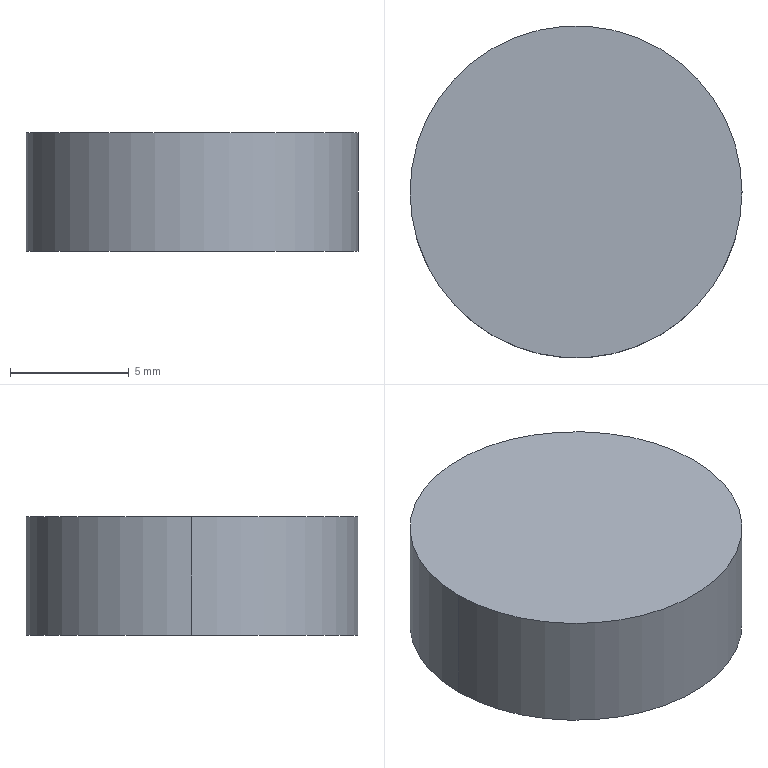Part | STEP file | PRODUCT_ID_90 | 1 solid | 11 faces | box 14 x 14 x 5 mm | volume 683.088 mm3 | plane 9 | cylinder 2 | commonest cylinder face diameters 14 x2
STEP:
#1=CARTESIAN_POINT('',(0.,0.,0.));
#2=DIRECTION('',(0.,0.,1.));
#3=DIRECTION('',(1.,0.,0.));
#4=AXIS2_PLACEMENT_3D('',#1,#2,#3);
#5=CARTESIAN_POINT('',(74.443,-2.5,-63.));
#6=VERTEX_POINT('',#5);
#7=CARTESIAN_POINT('',(75.887,0.,-63.));
#8=VERTEX_POINT('',#7);
#9=CARTESIAN_POINT('',(75.165,-1.25,-63.));
#10=DIRECTION('',(0.5,0.866,0.));
#11=VECTOR('',#10,1.);
#12=LINE('',#9,#11);
#13=CARTESIAN_POINT('',(73.,0.,-63.));
#14=DIRECTION('',(0.,0.,1.));
#15=DIRECTION('',(1.,0.,0.));
#16=AXIS2_PLACEMENT_3D('',#13,#14,#15);
#17=PLANE('',#16);
#18=CARTESIAN_POINT('',(2.165,-1.25));
#19=DIRECTION('',(0.5,0.866));
#20=VECTOR('',#19,1.);
#21=LINE('',#18,#20);
#22=(GEOMETRIC_REPRESENTATION_CONTEXT(2)PARAMETRIC_REPRESENTATION_CONTEXT()REPRESENTATION_CONTEXT('',''));
#23=DEFINITIONAL_REPRESENTATION('',(#21),#22);
#24=PCURVE('',#17,#23);
#25=CARTESIAN_POINT('',(75.165,-1.25,-65.));
#26=DIRECTION('',(-0.866,0.5,0.));
#27=DIRECTION('',(0.,0.,1.));
#28=AXIS2_PLACEMENT_3D('',#25,#26,#27);
#29=PLANE('',#28);
#30=CARTESIAN_POINT('',(2.,0.));
#31=DIRECTION('',(0.,1.));
#32=VECTOR('',#31,1.);
#33=LINE('',#30,#32);
#34=(GEOMETRIC_REPRESENTATION_CONTEXT(2)PARAMETRIC_REPRESENTATION_CONTEXT()REPRESENTATION_CONTEXT('',''));
#35=DEFINITIONAL_REPRESENTATION('',(#33),#34);
#36=PCURVE('',#29,#35);
#37=SURFACE_CURVE('',#12,(#24,#36),.PCURVE_S1.);
#38=EDGE_CURVE('',#6,#8,#37,.T.);
#39=ORIENTED_EDGE('',*,*,#38,.F.);
#40=CARTESIAN_POINT('',(71.557,-2.5,-63.));
#41=VERTEX_POINT('',#40);
#42=CARTESIAN_POINT('',(73.,-2.5,-63.));
#43=DIRECTION('',(1.,0.,0.));
#44=VECTOR('',#43,1.);
#45=LINE('',#42,#44);
#46=CARTESIAN_POINT('',(0.,-2.5));
#47=DIRECTION('',(1.,0.));
#48=VECTOR('',#47,1.);
#49=LINE('',#46,#48);
#50=(GEOMETRIC_REPRESENTATION_CONTEXT(2)PARAMETRIC_REPRESENTATION_CONTEXT()REPRESENTATION_CONTEXT('',''));
#51=DEFINITIONAL_REPRESENTATION('',(#49),#50);
#52=PCURVE('',#17,#51);
#53=CARTESIAN_POINT('',(73.,-2.5,-65.));
#54=DIRECTION('',(0.,1.,0.));
#55=DIRECTION('',(1.,0.,0.));
#56=AXIS2_PLACEMENT_3D('',#53,#54,#55);
#57=PLANE('',#56);
#58=CARTESIAN_POINT('',(0.,-2.));
#59=DIRECTION('',(1.,0.));
#60=VECTOR('',#59,1.);
#61=LINE('',#58,#60);
#62=(GEOMETRIC_REPRESENTATION_CONTEXT(2)PARAMETRIC_REPRESENTATION_CONTEXT()REPRESENTATION_CONTEXT('',''));
#63=DEFINITIONAL_REPRESENTATION('',(#61),#62);
#64=PCURVE('',#57,#63);
#65=SURFACE_CURVE('',#45,(#52,#64),.PCURVE_S1.);
#66=EDGE_CURVE('',#41,#6,#65,.T.);
#67=ORIENTED_EDGE('',*,*,#66,.F.);
#68=CARTESIAN_POINT('',(70.113,0.,-63.));
#69=VERTEX_POINT('',#68);
#70=CARTESIAN_POINT('',(70.835,-1.25,-63.));
#71=DIRECTION('',(0.5,-0.866,0.));
#72=VECTOR('',#71,1.);
#73=LINE('',#70,#72);
#74=CARTESIAN_POINT('',(-2.165,-1.25));
#75=DIRECTION('',(0.5,-0.866));
#76=VECTOR('',#75,1.);
#77=LINE('',#74,#76);
#78=(GEOMETRIC_REPRESENTATION_CONTEXT(2)PARAMETRIC_REPRESENTATION_CONTEXT()REPRESENTATION_CONTEXT('',''));
#79=DEFINITIONAL_REPRESENTATION('',(#77),#78);
#80=PCURVE('',#17,#79);
#81=CARTESIAN_POINT('',(70.835,-1.25,-65.));
#82=DIRECTION('',(0.866,0.5,0.));
#83=DIRECTION('',(0.,0.,-1.));
#84=AXIS2_PLACEMENT_3D('',#81,#82,#83);
#85=PLANE('',#84);
#86=CARTESIAN_POINT('',(-2.,0.));
#87=DIRECTION('',(0.,-1.));
#88=VECTOR('',#87,1.);
#89=LINE('',#86,#88);
#90=(GEOMETRIC_REPRESENTATION_CONTEXT(2)PARAMETRIC_REPRESENTATION_CONTEXT()REPRESENTATION_CONTEXT('',''));
#91=DEFINITIONAL_REPRESENTATION('',(#89),#90);
#92=PCURVE('',#85,#91);
#93=SURFACE_CURVE('',#73,(#80,#92),.PCURVE_S1.);
#94=EDGE_CURVE('',#69,#41,#93,.T.);
#95=ORIENTED_EDGE('',*,*,#94,.F.);
#96=CARTESIAN_POINT('',(71.557,2.5,-63.));
#97=VERTEX_POINT('',#96);
#98=CARTESIAN_POINT('',(70.835,1.25,-63.));
#99=DIRECTION('',(-0.5,-0.866,0.));
#100=VECTOR('',#99,1.);
#101=LINE('',#98,#100);
#102=CARTESIAN_POINT('',(-2.165,1.25));
#103=DIRECTION('',(-0.5,-0.866));
#104=VECTOR('',#103,1.);
#105=LINE('',#102,#104);
#106=(GEOMETRIC_REPRESENTATION_CONTEXT(2)PARAMETRIC_REPRESENTATION_CONTEXT()REPRESENTATION_CONTEXT('',''));
#107=DEFINITIONAL_REPRESENTATION('',(#105),#106);
#108=PCURVE('',#17,#107);
#109=CARTESIAN_POINT('',(70.835,1.25,-65.));
#110=DIRECTION('',(0.866,-0.5,0.));
#111=DIRECTION('',(0.,0.,-1.));
#112=AXIS2_PLACEMENT_3D('',#109,#110,#111);
#113=PLANE('',#112);
#114=CARTESIAN_POINT('',(-2.,0.));
#115=DIRECTION('',(0.,-1.));
#116=VECTOR('',#115,1.);
#117=LINE('',#114,#116);
#118=(GEOMETRIC_REPRESENTATION_CONTEXT(2)PARAMETRIC_REPRESENTATION_CONTEXT()REPRESENTATION_CONTEXT('',''));
#119=DEFINITIONAL_REPRESENTATION('',(#117),#118);
#120=PCURVE('',#113,#119);
#121=SURFACE_CURVE('',#101,(#108,#120),.PCURVE_S1.);
#122=EDGE_CURVE('',#97,#69,#121,.T.);
#123=ORIENTED_EDGE('',*,*,#122,.F.);
#124=CARTESIAN_POINT('',(74.443,2.5,-63.));
#125=VERTEX_POINT('',#124);
#126=CARTESIAN_POINT('',(73.,2.5,-63.));
#127=DIRECTION('',(-1.,0.,0.));
#128=VECTOR('',#127,1.);
#129=LINE('',#126,#128);
#130=CARTESIAN_POINT('',(0.,2.5));
#131=DIRECTION('',(-1.,0.));
#132=VECTOR('',#131,1.);
#133=LINE('',#130,#132);
#134=(GEOMETRIC_REPRESENTATION_CONTEXT(2)PARAMETRIC_REPRESENTATION_CONTEXT()REPRESENTATION_CONTEXT('',''));
#135=DEFINITIONAL_REPRESENTATION('',(#133),#134);
#136=PCURVE('',#17,#135);
#137=CARTESIAN_POINT('',(73.,2.5,-65.));
#138=DIRECTION('',(0.,-1.,0.));
#139=DIRECTION('',(0.,0.,-1.));
#140=AXIS2_PLACEMENT_3D('',#137,#138,#139);
#141=PLANE('',#140);
#142=CARTESIAN_POINT('',(-2.,0.));
#143=DIRECTION('',(0.,-1.));
#144=VECTOR('',#143,1.);
#145=LINE('',#142,#144);
#146=(GEOMETRIC_REPRESENTATION_CONTEXT(2)PARAMETRIC_REPRESENTATION_CONTEXT()REPRESENTATION_CONTEXT('',''));
#147=DEFINITIONAL_REPRESENTATION('',(#145),#146);
#148=PCURVE('',#141,#147);
#149=SURFACE_CURVE('',#129,(#136,#148),.PCURVE_S1.);
#150=EDGE_CURVE('',#125,#97,#149,.T.);
#151=ORIENTED_EDGE('',*,*,#150,.F.);
#152=CARTESIAN_POINT('',(75.165,1.25,-63.));
#153=DIRECTION('',(-0.5,0.866,0.));
#154=VECTOR('',#153,1.);
#155=LINE('',#152,#154);
#156=CARTESIAN_POINT('',(2.165,1.25));
#157=DIRECTION('',(-0.5,0.866));
#158=VECTOR('',#157,1.);
#159=LINE('',#156,#158);
#160=(GEOMETRIC_REPRESENTATION_CONTEXT(2)PARAMETRIC_REPRESENTATION_CONTEXT()REPRESENTATION_CONTEXT('',''));
#161=DEFINITIONAL_REPRESENTATION('',(#159),#160);
#162=PCURVE('',#17,#161);
#163=CARTESIAN_POINT('',(75.165,1.25,-65.));
#164=DIRECTION('',(-0.866,-0.5,0.));
#165=DIRECTION('',(-0.5,0.866,0.));
#166=AXIS2_PLACEMENT_3D('',#163,#164,#165);
#167=PLANE('',#166);
#168=CARTESIAN_POINT('',(0.,-2.));
#169=DIRECTION('',(1.,0.));
#170=VECTOR('',#169,1.);
#171=LINE('',#168,#170);
#172=(GEOMETRIC_REPRESENTATION_CONTEXT(2)PARAMETRIC_REPRESENTATION_CONTEXT()REPRESENTATION_CONTEXT('',''));
#173=DEFINITIONAL_REPRESENTATION('',(#171),#172);
#174=PCURVE('',#167,#173);
#175=SURFACE_CURVE('',#155,(#162,#174),.PCURVE_S1.);
#176=EDGE_CURVE('',#8,#125,#175,.T.);
#177=ORIENTED_EDGE('',*,*,#176,.F.);
#178=EDGE_LOOP('',(#39,#67,#95,#123,#151,#177));
#179=FACE_BOUND('',#178,.T.);
#180=ADVANCED_FACE('',(#179),#17,.F.);
#181=CARTESIAN_POINT('',(70.113,0.,-67.));
#182=VERTEX_POINT('',#181);
#183=CARTESIAN_POINT('',(70.113,0.,-65.));
#184=DIRECTION('',(0.,0.,-1.));
#185=VECTOR('',#184,1.);
#186=LINE('',#183,#185);
#187=CARTESIAN_POINT('',(0.,1.443));
#188=DIRECTION('',(1.,0.));
#189=VECTOR('',#188,1.);
#190=LINE('',#187,#189);
#191=(GEOMETRIC_REPRESENTATION_CONTEXT(2)PARAMETRIC_REPRESENTATION_CONTEXT()REPRESENTATION_CONTEXT('',''));
#192=DEFINITIONAL_REPRESENTATION('',(#190),#191);
#193=PCURVE('',#85,#192);
#194=CARTESIAN_POINT('',(0.,-1.443));
#195=DIRECTION('',(1.,0.));
#196=VECTOR('',#195,1.);
#197=LINE('',#194,#196);
#198=(GEOMETRIC_REPRESENTATION_CONTEXT(2)PARAMETRIC_REPRESENTATION_CONTEXT()REPRESENTATION_CONTEXT('',''));
#199=DEFINITIONAL_REPRESENTATION('',(#197),#198);
#200=PCURVE('',#113,#199);
#201=SURFACE_CURVE('',#186,(#193,#200),.PCURVE_S1.);
#202=EDGE_CURVE('',#69,#182,#201,.T.);
#203=ORIENTED_EDGE('',*,*,#202,.F.);
#204=ORIENTED_EDGE('',*,*,#94,.T.);
#205=CARTESIAN_POINT('',(71.557,-2.5,-67.));
#206=VERTEX_POINT('',#205);
#207=CARTESIAN_POINT('',(71.557,-2.5,-65.));
#208=DIRECTION('',(0.,0.,1.));
#209=VECTOR('',#208,1.);
#210=LINE('',#207,#209);
#211=CARTESIAN_POINT('',(0.,-1.443));
#212=DIRECTION('',(-1.,0.));
#213=VECTOR('',#212,1.);
#214=LINE('',#211,#213);
#215=(GEOMETRIC_REPRESENTATION_CONTEXT(2)PARAMETRIC_REPRESENTATION_CONTEXT()REPRESENTATION_CONTEXT('',''));
#216=DEFINITIONAL_REPRESENTATION('',(#214),#215);
#217=PCURVE('',#85,#216);
#218=CARTESIAN_POINT('',(-1.443,0.));
#219=DIRECTION('',(0.,-1.));
#220=VECTOR('',#219,1.);
#221=LINE('',#218,#220);
#222=(GEOMETRIC_REPRESENTATION_CONTEXT(2)PARAMETRIC_REPRESENTATION_CONTEXT()REPRESENTATION_CONTEXT('',''));
#223=DEFINITIONAL_REPRESENTATION('',(#221),#222);
#224=PCURVE('',#57,#223);
#225=SURFACE_CURVE('',#210,(#217,#224),.PCURVE_S1.);
#226=EDGE_CURVE('',#206,#41,#225,.T.);
#227=ORIENTED_EDGE('',*,*,#226,.F.);
#228=CARTESIAN_POINT('',(70.113,0.,-67.));
#229=DIRECTION('',(0.5,-0.866,0.));
#230=VECTOR('',#229,1.);
#231=LINE('',#228,#230);
#232=CARTESIAN_POINT('',(2.,1.443));
#233=DIRECTION('',(0.,-1.));
#234=VECTOR('',#233,1.);
#235=LINE('',#232,#234);
#236=(GEOMETRIC_REPRESENTATION_CONTEXT(2)PARAMETRIC_REPRESENTATION_CONTEXT()REPRESENTATION_CONTEXT('',''));
#237=DEFINITIONAL_REPRESENTATION('',(#235),#236);
#238=PCURVE('',#85,#237);
#239=CARTESIAN_POINT('',(73.,0.,-67.));
#240=DIRECTION('',(0.,0.,-1.));
#241=DIRECTION('',(0.,-1.,0.));
#242=AXIS2_PLACEMENT_3D('',#239,#240,#241);
#243=PLANE('',#242);
#244=CARTESIAN_POINT('',(0.,2.887));
#245=DIRECTION('',(0.866,-0.5));
#246=VECTOR('',#245,1.);
#247=LINE('',#244,#246);
#248=(GEOMETRIC_REPRESENTATION_CONTEXT(2)PARAMETRIC_REPRESENTATION_CONTEXT()REPRESENTATION_CONTEXT('',''));
#249=DEFINITIONAL_REPRESENTATION('',(#247),#248);
#250=PCURVE('',#243,#249);
#251=SURFACE_CURVE('',#231,(#238,#250),.PCURVE_S1.);
#252=EDGE_CURVE('',#182,#206,#251,.T.);
#253=ORIENTED_EDGE('',*,*,#252,.F.);
#254=EDGE_LOOP('',(#203,#204,#227,#253));
#255=FACE_BOUND('',#254,.T.);
#256=ADVANCED_FACE('',(#255),#85,.T.);
#257=ORIENTED_EDGE('',*,*,#226,.T.);
#258=ORIENTED_EDGE('',*,*,#66,.T.);
#259=CARTESIAN_POINT('',(74.443,-2.5,-67.));
#260=VERTEX_POINT('',#259);
#261=CARTESIAN_POINT('',(74.443,-2.5,-65.));
#262=DIRECTION('',(0.,0.,1.));
#263=VECTOR('',#262,1.);
#264=LINE('',#261,#263);
#265=CARTESIAN_POINT('',(1.443,0.));
#266=DIRECTION('',(0.,-1.));
#267=VECTOR('',#266,1.);
#268=LINE('',#265,#267);
#269=(GEOMETRIC_REPRESENTATION_CONTEXT(2)PARAMETRIC_REPRESENTATION_CONTEXT()REPRESENTATION_CONTEXT('',''));
#270=DEFINITIONAL_REPRESENTATION('',(#268),#269);
#271=PCURVE('',#57,#270);
#272=CARTESIAN_POINT('',(0.,-1.443));
#273=DIRECTION('',(1.,0.));
#274=VECTOR('',#273,1.);
#275=LINE('',#272,#274);
#276=(GEOMETRIC_REPRESENTATION_CONTEXT(2)PARAMETRIC_REPRESENTATION_CONTEXT()REPRESENTATION_CONTEXT('',''));
#277=DEFINITIONAL_REPRESENTATION('',(#275),#276);
#278=PCURVE('',#29,#277);
#279=SURFACE_CURVE('',#264,(#271,#278),.PCURVE_S1.);
#280=EDGE_CURVE('',#260,#6,#279,.T.);
#281=ORIENTED_EDGE('',*,*,#280,.F.);
#282=CARTESIAN_POINT('',(73.,-2.5,-67.));
#283=DIRECTION('',(1.,0.,0.));
#284=VECTOR('',#283,1.);
#285=LINE('',#282,#284);
#286=CARTESIAN_POINT('',(0.,2.));
#287=DIRECTION('',(1.,0.));
#288=VECTOR('',#287,1.);
#289=LINE('',#286,#288);
#290=(GEOMETRIC_REPRESENTATION_CONTEXT(2)PARAMETRIC_REPRESENTATION_CONTEXT()REPRESENTATION_CONTEXT('',''));
#291=DEFINITIONAL_REPRESENTATION('',(#289),#290);
#292=PCURVE('',#57,#291);
#293=CARTESIAN_POINT('',(2.5,0.));
#294=DIRECTION('',(0.,-1.));
#295=VECTOR('',#294,1.);
#296=LINE('',#293,#295);
#297=(GEOMETRIC_REPRESENTATION_CONTEXT(2)PARAMETRIC_REPRESENTATION_CONTEXT()REPRESENTATION_CONTEXT('',''));
#298=DEFINITIONAL_REPRESENTATION('',(#296),#297);
#299=PCURVE('',#243,#298);
#300=SURFACE_CURVE('',#285,(#292,#299),.PCURVE_S1.);
#301=EDGE_CURVE('',#206,#260,#300,.T.);
#302=ORIENTED_EDGE('',*,*,#301,.F.);
#303=EDGE_LOOP('',(#257,#258,#281,#302));
#304=FACE_BOUND('',#303,.T.);
#305=ADVANCED_FACE('',(#304),#57,.T.);
#306=ORIENTED_EDGE('',*,*,#280,.T.);
#307=ORIENTED_EDGE('',*,*,#38,.T.);
#308=CARTESIAN_POINT('',(75.887,0.,-67.));
#309=VERTEX_POINT('',#308);
#310=CARTESIAN_POINT('',(75.887,0.,-65.));
#311=DIRECTION('',(0.,0.,1.));
#312=VECTOR('',#311,1.);
#313=LINE('',#310,#312);
#314=CARTESIAN_POINT('',(0.,1.443));
#315=DIRECTION('',(1.,0.));
#316=VECTOR('',#315,1.);
#317=LINE('',#314,#316);
#318=(GEOMETRIC_REPRESENTATION_CONTEXT(2)PARAMETRIC_REPRESENTATION_CONTEXT()REPRESENTATION_CONTEXT('',''));
#319=DEFINITIONAL_REPRESENTATION('',(#317),#318);
#320=PCURVE('',#29,#319);
#321=CARTESIAN_POINT('',(-1.443,0.));
#322=DIRECTION('',(0.,-1.));
#323=VECTOR('',#322,1.);
#324=LINE('',#321,#323);
#325=(GEOMETRIC_REPRESENTATION_CONTEXT(2)PARAMETRIC_REPRESENTATION_CONTEXT()REPRESENTATION_CONTEXT('',''));
#326=DEFINITIONAL_REPRESENTATION('',(#324),#325);
#327=PCURVE('',#167,#326);
#328=SURFACE_CURVE('',#313,(#320,#327),.PCURVE_S1.);
#329=EDGE_CURVE('',#309,#8,#328,.T.);
#330=ORIENTED_EDGE('',*,*,#329,.F.);
#331=CARTESIAN_POINT('',(74.443,-2.5,-67.));
#332=DIRECTION('',(0.5,0.866,0.));
#333=VECTOR('',#332,1.);
#334=LINE('',#331,#333);
#335=CARTESIAN_POINT('',(-2.,-1.443));
#336=DIRECTION('',(0.,1.));
#337=VECTOR('',#336,1.);
#338=LINE('',#335,#337);
#339=(GEOMETRIC_REPRESENTATION_CONTEXT(2)PARAMETRIC_REPRESENTATION_CONTEXT()REPRESENTATION_CONTEXT('',''));
#340=DEFINITIONAL_REPRESENTATION('',(#338),#339);
#341=PCURVE('',#29,#340);
#342=CARTESIAN_POINT('',(2.5,-1.443));
#343=DIRECTION('',(-0.866,-0.5));
#344=VECTOR('',#343,1.);
#345=LINE('',#342,#344);
#346=(GEOMETRIC_REPRESENTATION_CONTEXT(2)PARAMETRIC_REPRESENTATION_CONTEXT()REPRESENTATION_CONTEXT('',''));
#347=DEFINITIONAL_REPRESENTATION('',(#345),#346);
#348=PCURVE('',#243,#347);
#349=SURFACE_CURVE('',#334,(#341,#348),.PCURVE_S1.);
#350=EDGE_CURVE('',#260,#309,#349,.T.);
#351=ORIENTED_EDGE('',*,*,#350,.F.);
#352=EDGE_LOOP('',(#306,#307,#330,#351));
#353=FACE_BOUND('',#352,.T.);
#354=ADVANCED_FACE('',(#353),#29,.T.);
#355=ORIENTED_EDGE('',*,*,#329,.T.);
#356=ORIENTED_EDGE('',*,*,#176,.T.);
#357=CARTESIAN_POINT('',(74.443,2.5,-67.));
#358=VERTEX_POINT('',#357);
#359=CARTESIAN_POINT('',(74.443,2.5,-65.));
#360=DIRECTION('',(0.,0.,1.));
#361=VECTOR('',#360,1.);
#362=LINE('',#359,#361);
#363=CARTESIAN_POINT('',(1.443,0.));
#364=DIRECTION('',(0.,-1.));
#365=VECTOR('',#364,1.);
#366=LINE('',#363,#365);
#367=(GEOMETRIC_REPRESENTATION_CONTEXT(2)PARAMETRIC_REPRESENTATION_CONTEXT()REPRESENTATION_CONTEXT('',''));
#368=DEFINITIONAL_REPRESENTATION('',(#366),#367);
#369=PCURVE('',#167,#368);
#370=CARTESIAN_POINT('',(0.,1.443));
#371=DIRECTION('',(-1.,0.));
#372=VECTOR('',#371,1.);
#373=LINE('',#370,#372);
#374=(GEOMETRIC_REPRESENTATION_CONTEXT(2)PARAMETRIC_REPRESENTATION_CONTEXT()REPRESENTATION_CONTEXT('',''));
#375=DEFINITIONAL_REPRESENTATION('',(#373),#374);
#376=PCURVE('',#141,#375);
#377=SURFACE_CURVE('',#362,(#369,#376),.PCURVE_S1.);
#378=EDGE_CURVE('',#358,#125,#377,.T.);
#379=ORIENTED_EDGE('',*,*,#378,.F.);
#380=CARTESIAN_POINT('',(75.887,0.,-67.));
#381=DIRECTION('',(-0.5,0.866,0.));
#382=VECTOR('',#381,1.);
#383=LINE('',#380,#382);
#384=CARTESIAN_POINT('',(-1.443,2.));
#385=DIRECTION('',(1.,0.));
#386=VECTOR('',#385,1.);
#387=LINE('',#384,#386);
#388=(GEOMETRIC_REPRESENTATION_CONTEXT(2)PARAMETRIC_REPRESENTATION_CONTEXT()REPRESENTATION_CONTEXT('',''));
#389=DEFINITIONAL_REPRESENTATION('',(#387),#388);
#390=PCURVE('',#167,#389);
#391=CARTESIAN_POINT('',(0.,-2.887));
#392=DIRECTION('',(-0.866,0.5));
#393=VECTOR('',#392,1.);
#394=LINE('',#391,#393);
#395=(GEOMETRIC_REPRESENTATION_CONTEXT(2)PARAMETRIC_REPRESENTATION_CONTEXT()REPRESENTATION_CONTEXT('',''));
#396=DEFINITIONAL_REPRESENTATION('',(#394),#395);
#397=PCURVE('',#243,#396);
#398=SURFACE_CURVE('',#383,(#390,#397),.PCURVE_S1.);
#399=EDGE_CURVE('',#309,#358,#398,.T.);
#400=ORIENTED_EDGE('',*,*,#399,.F.);
#401=EDGE_LOOP('',(#355,#356,#379,#400));
#402=FACE_BOUND('',#401,.T.);
#403=ADVANCED_FACE('',(#402),#167,.T.);
#404=ORIENTED_EDGE('',*,*,#378,.T.);
#405=ORIENTED_EDGE('',*,*,#150,.T.);
#406=CARTESIAN_POINT('',(71.557,2.5,-67.));
#407=VERTEX_POINT('',#406);
#408=CARTESIAN_POINT('',(71.557,2.5,-65.));
#409=DIRECTION('',(0.,0.,1.));
#410=VECTOR('',#409,1.);
#411=LINE('',#408,#410);
#412=CARTESIAN_POINT('',(0.,-1.443));
#413=DIRECTION('',(-1.,0.));
#414=VECTOR('',#413,1.);
#415=LINE('',#412,#414);
#416=(GEOMETRIC_REPRESENTATION_CONTEXT(2)PARAMETRIC_REPRESENTATION_CONTEXT()REPRESENTATION_CONTEXT('',''));
#417=DEFINITIONAL_REPRESENTATION('',(#415),#416);
#418=PCURVE('',#141,#417);
#419=CARTESIAN_POINT('',(0.,1.443));
#420=DIRECTION('',(-1.,0.));
#421=VECTOR('',#420,1.);
#422=LINE('',#419,#421);
#423=(GEOMETRIC_REPRESENTATION_CONTEXT(2)PARAMETRIC_REPRESENTATION_CONTEXT()REPRESENTATION_CONTEXT('',''));
#424=DEFINITIONAL_REPRESENTATION('',(#422),#423);
#425=PCURVE('',#113,#424);
#426=SURFACE_CURVE('',#411,(#418,#425),.PCURVE_S1.);
#427=EDGE_CURVE('',#407,#97,#426,.T.);
#428=ORIENTED_EDGE('',*,*,#427,.F.);
#429=CARTESIAN_POINT('',(73.,2.5,-67.));
#430=DIRECTION('',(-1.,0.,0.));
#431=VECTOR('',#430,1.);
#432=LINE('',#429,#431);
#433=CARTESIAN_POINT('',(2.,0.));
#434=DIRECTION('',(0.,-1.));
#435=VECTOR('',#434,1.);
#436=LINE('',#433,#435);
#437=(GEOMETRIC_REPRESENTATION_CONTEXT(2)PARAMETRIC_REPRESENTATION_CONTEXT()REPRESENTATION_CONTEXT('',''));
#438=DEFINITIONAL_REPRESENTATION('',(#436),#437);
#439=PCURVE('',#141,#438);
#440=CARTESIAN_POINT('',(-2.5,0.));
#441=DIRECTION('',(0.,1.));
#442=VECTOR('',#441,1.);
#443=LINE('',#440,#442);
#444=(GEOMETRIC_REPRESENTATION_CONTEXT(2)PARAMETRIC_REPRESENTATION_CONTEXT()REPRESENTATION_CONTEXT('',''));
#445=DEFINITIONAL_REPRESENTATION('',(#443),#444);
#446=PCURVE('',#243,#445);
#447=SURFACE_CURVE('',#432,(#439,#446),.PCURVE_S1.);
#448=EDGE_CURVE('',#358,#407,#447,.T.);
#449=ORIENTED_EDGE('',*,*,#448,.F.);
#450=EDGE_LOOP('',(#404,#405,#428,#449));
#451=FACE_BOUND('',#450,.T.);
#452=ADVANCED_FACE('',(#451),#141,.T.);
#453=ORIENTED_EDGE('',*,*,#427,.T.);
#454=ORIENTED_EDGE('',*,*,#122,.T.);
#455=ORIENTED_EDGE('',*,*,#202,.T.);
#456=CARTESIAN_POINT('',(71.557,2.5,-67.));
#457=DIRECTION('',(-0.5,-0.866,0.));
#458=VECTOR('',#457,1.);
#459=LINE('',#456,#458);
#460=CARTESIAN_POINT('',(2.,1.443));
#461=DIRECTION('',(0.,-1.));
#462=VECTOR('',#461,1.);
#463=LINE('',#460,#462);
#464=(GEOMETRIC_REPRESENTATION_CONTEXT(2)PARAMETRIC_REPRESENTATION_CONTEXT()REPRESENTATION_CONTEXT('',''));
#465=DEFINITIONAL_REPRESENTATION('',(#463),#464);
#466=PCURVE('',#113,#465);
#467=CARTESIAN_POINT('',(-2.5,1.443));
#468=DIRECTION('',(0.866,0.5));
#469=VECTOR('',#468,1.);
#470=LINE('',#467,#469);
#471=(GEOMETRIC_REPRESENTATION_CONTEXT(2)PARAMETRIC_REPRESENTATION_CONTEXT()REPRESENTATION_CONTEXT('',''));
#472=DEFINITIONAL_REPRESENTATION('',(#470),#471);
#473=PCURVE('',#243,#472);
#474=SURFACE_CURVE('',#459,(#466,#473),.PCURVE_S1.);
#475=EDGE_CURVE('',#407,#182,#474,.T.);
#476=ORIENTED_EDGE('',*,*,#475,.F.);
#477=EDGE_LOOP('',(#453,#454,#455,#476));
#478=FACE_BOUND('',#477,.T.);
#479=ADVANCED_FACE('',(#478),#113,.T.);
#480=ORIENTED_EDGE('',*,*,#448,.T.);
#481=ORIENTED_EDGE('',*,*,#475,.T.);
#482=ORIENTED_EDGE('',*,*,#252,.T.);
#483=ORIENTED_EDGE('',*,*,#301,.T.);
#484=ORIENTED_EDGE('',*,*,#350,.T.);
#485=ORIENTED_EDGE('',*,*,#399,.T.);
#486=EDGE_LOOP('',(#480,#481,#482,#483,#484,#485));
#487=FACE_BOUND('',#486,.T.);
#488=CARTESIAN_POINT('',(80.,0.,-67.));
#489=VERTEX_POINT('',#488);
#490=CARTESIAN_POINT('',(66.,0.,-67.));
#491=VERTEX_POINT('',#490);
#492=CARTESIAN_POINT('',(73.,0.,-67.));
#493=DIRECTION('',(0.,0.,1.));
#494=DIRECTION('',(1.,0.,0.));
#495=AXIS2_PLACEMENT_3D('',#492,#493,#494);
#496=CIRCLE('',#495,7.);
#497=CARTESIAN_POINT('',(0.,-7.));
#498=CARTESIAN_POINT('',(-12.124,-7.));
#499=CARTESIAN_POINT('',(-6.062,3.5));
#500=CARTESIAN_POINT('',(0.,14.));
#501=CARTESIAN_POINT('',(6.062,3.5));
#502=CARTESIAN_POINT('',(12.124,-7.));
#503=CARTESIAN_POINT('',(0.,-7.));
#504=(BOUNDED_CURVE()B_SPLINE_CURVE(2,(#497,#498,#499,#500,#501,#502,#503),.UNSPECIFIED.,.T.,.F.)B_SPLINE_CURVE_WITH_KNOTS((1,2,2,2,2,1),(-2.094,0.,2.094,4.189,6.283,8.378),.UNSPECIFIED.)CURVE()GEOMETRIC_REPRESENTATION_ITEM()RATIONAL_B_SPLINE_CURVE((1.,0.5,1.,0.5,1.,0.5,1.))REPRESENTATION_ITEM(''));
#505=(GEOMETRIC_REPRESENTATION_CONTEXT(2)PARAMETRIC_REPRESENTATION_CONTEXT()REPRESENTATION_CONTEXT('',''));
#506=DEFINITIONAL_REPRESENTATION('',(#504),#505);
#507=PCURVE('',#243,#506);
#508=CARTESIAN_POINT('',(73.,0.,-64.5));
#509=DIRECTION('',(0.,0.,1.));
#510=DIRECTION('',(1.,0.,0.));
#511=AXIS2_PLACEMENT_3D('',#508,#509,#510);
#512=CYLINDRICAL_SURFACE('',#511,7.);
#513=CARTESIAN_POINT('',(0.,-2.5));
#514=DIRECTION('',(1.,0.));
#515=VECTOR('',#514,1.);
#516=LINE('',#513,#515);
#517=(GEOMETRIC_REPRESENTATION_CONTEXT(2)PARAMETRIC_REPRESENTATION_CONTEXT()REPRESENTATION_CONTEXT('',''));
#518=DEFINITIONAL_REPRESENTATION('',(#516),#517);
#519=PCURVE('',#512,#518);
#520=SURFACE_CURVE('',#496,(#507,#519),.PCURVE_S1.);
#521=EDGE_CURVE('',#489,#491,#520,.T.);
#522=ORIENTED_EDGE('',*,*,#521,.F.);
#523=CARTESIAN_POINT('',(73.,0.,-67.));
#524=DIRECTION('',(0.,0.,1.));
#525=DIRECTION('',(1.,0.,0.));
#526=AXIS2_PLACEMENT_3D('',#523,#524,#525);
#527=CIRCLE('',#526,7.);
#528=CARTESIAN_POINT('',(0.,-7.));
#529=CARTESIAN_POINT('',(-12.124,-7.));
#530=CARTESIAN_POINT('',(-6.062,3.5));
#531=CARTESIAN_POINT('',(0.,14.));
#532=CARTESIAN_POINT('',(6.062,3.5));
#533=CARTESIAN_POINT('',(12.124,-7.));
#534=CARTESIAN_POINT('',(0.,-7.));
#535=(BOUNDED_CURVE()B_SPLINE_CURVE(2,(#528,#529,#530,#531,#532,#533,#534),.UNSPECIFIED.,.T.,.F.)B_SPLINE_CURVE_WITH_KNOTS((1,2,2,2,2,1),(-2.094,0.,2.094,4.189,6.283,8.378),.UNSPECIFIED.)CURVE()GEOMETRIC_REPRESENTATION_ITEM()RATIONAL_B_SPLINE_CURVE((1.,0.5,1.,0.5,1.,0.5,1.))REPRESENTATION_ITEM(''));
#536=(GEOMETRIC_REPRESENTATION_CONTEXT(2)PARAMETRIC_REPRESENTATION_CONTEXT()REPRESENTATION_CONTEXT('',''));
#537=DEFINITIONAL_REPRESENTATION('',(#535),#536);
#538=PCURVE('',#243,#537);
#539=CARTESIAN_POINT('',(73.,0.,-64.5));
#540=DIRECTION('',(0.,0.,1.));
#541=DIRECTION('',(1.,0.,0.));
#542=AXIS2_PLACEMENT_3D('',#539,#540,#541);
#543=CYLINDRICAL_SURFACE('',#542,7.);
#544=CARTESIAN_POINT('',(0.,-2.5));
#545=DIRECTION('',(1.,0.));
#546=VECTOR('',#545,1.);
#547=LINE('',#544,#546);
#548=(GEOMETRIC_REPRESENTATION_CONTEXT(2)PARAMETRIC_REPRESENTATION_CONTEXT()REPRESENTATION_CONTEXT('',''));
#549=DEFINITIONAL_REPRESENTATION('',(#547),#548);
#550=PCURVE('',#543,#549);
#551=SURFACE_CURVE('',#527,(#538,#550),.PCURVE_S1.);
#552=EDGE_CURVE('',#491,#489,#551,.T.);
#553=ORIENTED_EDGE('',*,*,#552,.F.);
#554=EDGE_LOOP('',(#522,#553));
#555=FACE_BOUND('',#554,.T.);
#556=ADVANCED_FACE('',(#487,#555),#243,.T.);
#557=CARTESIAN_POINT('',(66.,0.,-62.));
#558=VERTEX_POINT('',#557);
#559=CARTESIAN_POINT('',(66.,0.,-64.5));
#560=DIRECTION('',(0.,0.,1.));
#561=VECTOR('',#560,1.);
#562=LINE('',#559,#561);
#563=CARTESIAN_POINT('',(3.142,0.));
#564=DIRECTION('',(0.,1.));
#565=VECTOR('',#564,1.);
#566=LINE('',#563,#565);
#567=(GEOMETRIC_REPRESENTATION_CONTEXT(2)PARAMETRIC_REPRESENTATION_CONTEXT()REPRESENTATION_CONTEXT('',''));
#568=DEFINITIONAL_REPRESENTATION('',(#566),#567);
#569=PCURVE('',#543,#568);
#570=CARTESIAN_POINT('',(3.142,0.));
#571=DIRECTION('',(0.,1.));
#572=VECTOR('',#571,1.);
#573=LINE('',#570,#572);
#574=(GEOMETRIC_REPRESENTATION_CONTEXT(2)PARAMETRIC_REPRESENTATION_CONTEXT()REPRESENTATION_CONTEXT('',''));
#575=DEFINITIONAL_REPRESENTATION('',(#573),#574);
#576=PCURVE('',#512,#575);
#577=SURFACE_CURVE('',#562,(#569,#576),.PCURVE_S1.);
#578=EDGE_CURVE('',#491,#558,#577,.T.);
#579=ORIENTED_EDGE('',*,*,#578,.F.);
#580=ORIENTED_EDGE('',*,*,#552,.T.);
#581=CARTESIAN_POINT('',(80.,0.,-62.));
#582=VERTEX_POINT('',#581);
#583=CARTESIAN_POINT('',(80.,0.,-64.5));
#584=DIRECTION('',(0.,0.,1.));
#585=VECTOR('',#584,1.);
#586=LINE('',#583,#585);
#587=CARTESIAN_POINT('',(6.283,0.));
#588=DIRECTION('',(0.,1.));
#589=VECTOR('',#588,1.);
#590=LINE('',#587,#589);
#591=(GEOMETRIC_REPRESENTATION_CONTEXT(2)PARAMETRIC_REPRESENTATION_CONTEXT()REPRESENTATION_CONTEXT('',''));
#592=DEFINITIONAL_REPRESENTATION('',(#590),#591);
#593=PCURVE('',#543,#592);
#594=CARTESIAN_POINT('',(0.,0.));
#595=DIRECTION('',(0.,1.));
#596=VECTOR('',#595,1.);
#597=LINE('',#594,#596);
#598=(GEOMETRIC_REPRESENTATION_CONTEXT(2)PARAMETRIC_REPRESENTATION_CONTEXT()REPRESENTATION_CONTEXT('',''));
#599=DEFINITIONAL_REPRESENTATION('',(#597),#598);
#600=PCURVE('',#512,#599);
#601=SURFACE_CURVE('',#586,(#593,#600),.PCURVE_S1.);
#602=EDGE_CURVE('',#489,#582,#601,.T.);
#603=ORIENTED_EDGE('',*,*,#602,.T.);
#604=CARTESIAN_POINT('',(73.,0.,-62.));
#605=DIRECTION('',(0.,0.,1.));
#606=DIRECTION('',(1.,0.,0.));
#607=AXIS2_PLACEMENT_3D('',#604,#605,#606);
#608=CIRCLE('',#607,7.);
#609=CARTESIAN_POINT('',(0.,2.5));
#610=DIRECTION('',(1.,0.));
#611=VECTOR('',#610,1.);
#612=LINE('',#609,#611);
#613=(GEOMETRIC_REPRESENTATION_CONTEXT(2)PARAMETRIC_REPRESENTATION_CONTEXT()REPRESENTATION_CONTEXT('',''));
#614=DEFINITIONAL_REPRESENTATION('',(#612),#613);
#615=PCURVE('',#543,#614);
#616=CARTESIAN_POINT('',(73.,0.,-62.));
#617=DIRECTION('',(0.,0.,1.));
#618=DIRECTION('',(1.,0.,0.));
#619=AXIS2_PLACEMENT_3D('',#616,#617,#618);
#620=PLANE('',#619);
#621=CARTESIAN_POINT('',(0.,0.));
#622=DIRECTION('',(1.,0.));
#623=AXIS2_PLACEMENT_2D('',#621,#622);
#624=CIRCLE('',#623,7.);
#625=(GEOMETRIC_REPRESENTATION_CONTEXT(2)PARAMETRIC_REPRESENTATION_CONTEXT()REPRESENTATION_CONTEXT('',''));
#626=DEFINITIONAL_REPRESENTATION('',(#624),#625);
#627=PCURVE('',#620,#626);
#628=SURFACE_CURVE('',#608,(#615,#627),.PCURVE_S1.);
#629=EDGE_CURVE('',#558,#582,#628,.T.);
#630=ORIENTED_EDGE('',*,*,#629,.F.);
#631=EDGE_LOOP('',(#579,#580,#603,#630));
#632=FACE_BOUND('',#631,.T.);
#633=ADVANCED_FACE('',(#632),#543,.T.);
#634=CARTESIAN_POINT('',(73.,0.,-62.));
#635=DIRECTION('',(0.,0.,1.));
#636=DIRECTION('',(1.,0.,0.));
#637=AXIS2_PLACEMENT_3D('',#634,#635,#636);
#638=CIRCLE('',#637,7.);
#639=CARTESIAN_POINT('',(0.,0.));
#640=DIRECTION('',(1.,0.));
#641=AXIS2_PLACEMENT_2D('',#639,#640);
#642=CIRCLE('',#641,7.);
#643=(GEOMETRIC_REPRESENTATION_CONTEXT(2)PARAMETRIC_REPRESENTATION_CONTEXT()REPRESENTATION_CONTEXT('',''));
#644=DEFINITIONAL_REPRESENTATION('',(#642),#643);
#645=PCURVE('',#620,#644);
#646=CARTESIAN_POINT('',(0.,2.5));
#647=DIRECTION('',(1.,0.));
#648=VECTOR('',#647,1.);
#649=LINE('',#646,#648);
#650=(GEOMETRIC_REPRESENTATION_CONTEXT(2)PARAMETRIC_REPRESENTATION_CONTEXT()REPRESENTATION_CONTEXT('',''));
#651=DEFINITIONAL_REPRESENTATION('',(#649),#650);
#652=PCURVE('',#512,#651);
#653=SURFACE_CURVE('',#638,(#645,#652),.PCURVE_S1.);
#654=EDGE_CURVE('',#582,#558,#653,.T.);
#655=ORIENTED_EDGE('',*,*,#654,.T.);
#656=ORIENTED_EDGE('',*,*,#629,.T.);
#657=EDGE_LOOP('',(#655,#656));
#658=FACE_BOUND('',#657,.T.);
#659=ADVANCED_FACE('',(#658),#620,.T.);
#660=ORIENTED_EDGE('',*,*,#521,.T.);
#661=ORIENTED_EDGE('',*,*,#578,.T.);
#662=ORIENTED_EDGE('',*,*,#654,.F.);
#663=ORIENTED_EDGE('',*,*,#602,.F.);
#664=EDGE_LOOP('',(#660,#661,#662,#663));
#665=FACE_BOUND('',#664,.T.);
#666=ADVANCED_FACE('',(#665),#512,.T.);
#667=CLOSED_SHELL('',(#180,#256,#305,#354,#403,#452,#479,#556,#633,#659,#666));
#668=MANIFOLD_SOLID_BREP('',#667);
#669=(LENGTH_UNIT()NAMED_UNIT(*)SI_UNIT(.MILLI.,.METRE.));
#670=UNCERTAINTY_MEASURE_WITH_UNIT(LENGTH_MEASURE(0.0000001),#669,'','');
#671=(NAMED_UNIT(*)PLANE_ANGLE_UNIT()SI_UNIT($,.RADIAN.));
#672=(NAMED_UNIT(*)SI_UNIT($,.STERADIAN.)SOLID_ANGLE_UNIT());
#673=(GEOMETRIC_REPRESENTATION_CONTEXT(3)GLOBAL_UNCERTAINTY_ASSIGNED_CONTEXT((#670))GLOBAL_UNIT_ASSIGNED_CONTEXT((#669,#671,#672))REPRESENTATION_CONTEXT('',''));
#674=ADVANCED_BREP_SHAPE_REPRESENTATION('',(#4,#668),#673);